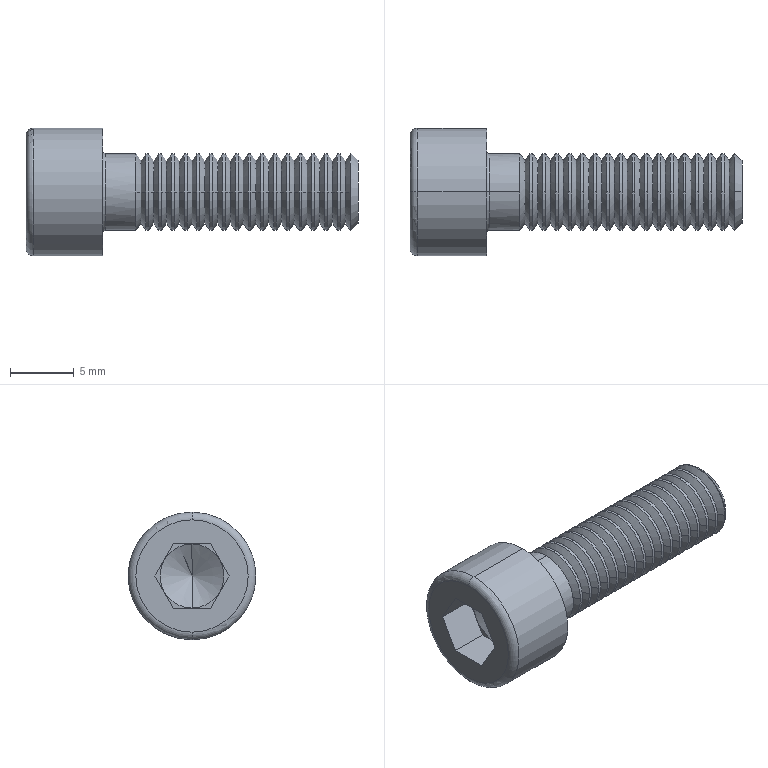Part | STEP file | socket head cap screw 4762_din_ISO 4762 M6 x 20 --- 20S | 1 solid | 129 faces | box 26 x 10 x 10 mm | volume 892.13 mm3 | cone 72 | cylinder 38 | plane 15 | torus 4 | commonest cylinder face diameters 6 x36 10 x2